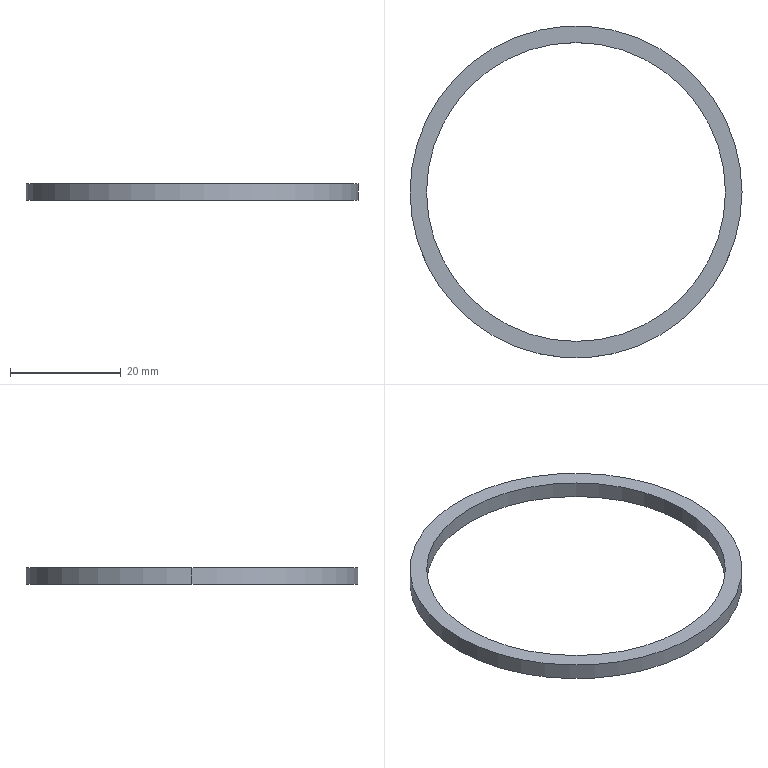Part | SolidWorks | features Extrusion 1 | 1 solid | 6 faces | box 60 x 60 x 3 mm | volume 1612 mm3 | cylinder 4 | plane 2 | commonest cylinder face diameters 54 x2 60 x2
STEP:
#1=CARTESIAN_POINT('',(-27.,0.,3.));
#2=VERTEX_POINT('',#1);
#3=CARTESIAN_POINT('',(27.,0.,3.));
#4=VERTEX_POINT('',#3);
#5=CARTESIAN_POINT('',(0.,0.,3.));
#6=DIRECTION('',(0.,0.,1.));
#7=DIRECTION('',(1.,0.,0.));
#8=AXIS2_PLACEMENT_3D('',#5,#6,#7);
#9=CIRCLE('',#8,27.);
#10=EDGE_CURVE('',#2,#4,#9,.T.);
#11=ORIENTED_EDGE('',*,*,#10,.T.);
#12=CARTESIAN_POINT('',(27.,0.,0.));
#13=VERTEX_POINT('',#12);
#14=CARTESIAN_POINT('',(27.,0.,3.));
#15=DIRECTION('',(0.,0.,-1.));
#16=VECTOR('',#15,1000.);
#17=LINE('',#14,#16);
#18=EDGE_CURVE('',#4,#13,#17,.T.);
#19=ORIENTED_EDGE('',*,*,#18,.T.);
#20=CARTESIAN_POINT('',(-27.,0.,0.));
#21=VERTEX_POINT('',#20);
#22=CARTESIAN_POINT('',(0.,0.,0.));
#23=DIRECTION('',(0.,0.,1.));
#24=DIRECTION('',(1.,0.,0.));
#25=AXIS2_PLACEMENT_3D('',#22,#23,#24);
#26=CIRCLE('',#25,27.);
#27=EDGE_CURVE('',#21,#13,#26,.T.);
#28=ORIENTED_EDGE('',*,*,#27,.F.);
#29=CARTESIAN_POINT('',(-27.,0.,3.));
#30=DIRECTION('',(0.,0.,-1.));
#31=VECTOR('',#30,1000.);
#32=LINE('',#29,#31);
#33=EDGE_CURVE('',#2,#21,#32,.T.);
#34=ORIENTED_EDGE('',*,*,#33,.F.);
#35=EDGE_LOOP('',(#11,#19,#28,#34));
#36=FACE_OUTER_BOUND('',#35,.T.);
#37=CARTESIAN_POINT('',(0.,0.,3.));
#38=DIRECTION('',(0.,0.,-1.));
#39=DIRECTION('',(-1.,0.,0.));
#40=AXIS2_PLACEMENT_3D('',#37,#38,#39);
#41=CYLINDRICAL_SURFACE('',#40,27.);
#42=ADVANCED_FACE('',(#36),#41,.F.);
#43=CARTESIAN_POINT('',(30.,0.,3.));
#44=VERTEX_POINT('',#43);
#45=CARTESIAN_POINT('',(-30.,0.,3.));
#46=VERTEX_POINT('',#45);
#47=CARTESIAN_POINT('',(0.,0.,3.));
#48=DIRECTION('',(0.,0.,1.));
#49=DIRECTION('',(1.,0.,0.));
#50=AXIS2_PLACEMENT_3D('',#47,#48,#49);
#51=CIRCLE('',#50,30.);
#52=EDGE_CURVE('',#44,#46,#51,.T.);
#53=ORIENTED_EDGE('',*,*,#52,.F.);
#54=CARTESIAN_POINT('',(30.,0.,0.));
#55=VERTEX_POINT('',#54);
#56=CARTESIAN_POINT('',(30.,0.,3.));
#57=DIRECTION('',(0.,0.,-1.));
#58=VECTOR('',#57,1000.);
#59=LINE('',#56,#58);
#60=EDGE_CURVE('',#44,#55,#59,.T.);
#61=ORIENTED_EDGE('',*,*,#60,.T.);
#62=CARTESIAN_POINT('',(-30.,0.,0.));
#63=VERTEX_POINT('',#62);
#64=CARTESIAN_POINT('',(0.,0.,0.));
#65=DIRECTION('',(0.,0.,1.));
#66=DIRECTION('',(1.,0.,0.));
#67=AXIS2_PLACEMENT_3D('',#64,#65,#66);
#68=CIRCLE('',#67,30.);
#69=EDGE_CURVE('',#55,#63,#68,.T.);
#70=ORIENTED_EDGE('',*,*,#69,.T.);
#71=CARTESIAN_POINT('',(-30.,0.,3.));
#72=DIRECTION('',(0.,0.,-1.));
#73=VECTOR('',#72,1000.);
#74=LINE('',#71,#73);
#75=EDGE_CURVE('',#46,#63,#74,.T.);
#76=ORIENTED_EDGE('',*,*,#75,.F.);
#77=EDGE_LOOP('',(#53,#61,#70,#76));
#78=FACE_OUTER_BOUND('',#77,.T.);
#79=CARTESIAN_POINT('',(0.,0.,3.));
#80=DIRECTION('',(0.,0.,-1.));
#81=DIRECTION('',(-1.,0.,0.));
#82=AXIS2_PLACEMENT_3D('',#79,#80,#81);
#83=CYLINDRICAL_SURFACE('',#82,30.);
#84=ADVANCED_FACE('',(#78),#83,.T.);
#85=CARTESIAN_POINT('',(0.,0.,3.));
#86=DIRECTION('',(0.,0.,1.));
#87=DIRECTION('',(1.,0.,0.));
#88=AXIS2_PLACEMENT_3D('',#85,#86,#87);
#89=CIRCLE('',#88,30.);
#90=EDGE_CURVE('',#46,#44,#89,.T.);
#91=ORIENTED_EDGE('',*,*,#90,.T.);
#92=ORIENTED_EDGE('',*,*,#52,.T.);
#93=EDGE_LOOP('',(#91,#92));
#94=FACE_OUTER_BOUND('',#93,.T.);
#95=ORIENTED_EDGE('',*,*,#10,.F.);
#96=CARTESIAN_POINT('',(0.,0.,3.));
#97=DIRECTION('',(0.,0.,1.));
#98=DIRECTION('',(1.,0.,0.));
#99=AXIS2_PLACEMENT_3D('',#96,#97,#98);
#100=CIRCLE('',#99,27.);
#101=EDGE_CURVE('',#4,#2,#100,.T.);
#102=ORIENTED_EDGE('',*,*,#101,.F.);
#103=EDGE_LOOP('',(#95,#102));
#104=FACE_BOUND('',#103,.T.);
#105=CARTESIAN_POINT('',(0.,0.,3.));
#106=DIRECTION('',(0.,0.,1.));
#107=DIRECTION('',(1.,0.,0.));
#108=AXIS2_PLACEMENT_3D('',#105,#106,#107);
#109=PLANE('',#108);
#110=ADVANCED_FACE('',(#94,#104),#109,.T.);
#111=CARTESIAN_POINT('',(0.,0.,0.));
#112=DIRECTION('',(0.,0.,1.));
#113=DIRECTION('',(1.,0.,0.));
#114=AXIS2_PLACEMENT_3D('',#111,#112,#113);
#115=CIRCLE('',#114,30.);
#116=EDGE_CURVE('',#63,#55,#115,.T.);
#117=ORIENTED_EDGE('',*,*,#116,.F.);
#118=ORIENTED_EDGE('',*,*,#69,.F.);
#119=EDGE_LOOP('',(#117,#118));
#120=FACE_OUTER_BOUND('',#119,.T.);
#121=ORIENTED_EDGE('',*,*,#27,.T.);
#122=CARTESIAN_POINT('',(0.,0.,0.));
#123=DIRECTION('',(0.,0.,1.));
#124=DIRECTION('',(1.,0.,0.));
#125=AXIS2_PLACEMENT_3D('',#122,#123,#124);
#126=CIRCLE('',#125,27.);
#127=EDGE_CURVE('',#13,#21,#126,.T.);
#128=ORIENTED_EDGE('',*,*,#127,.T.);
#129=EDGE_LOOP('',(#121,#128));
#130=FACE_BOUND('',#129,.T.);
#131=CARTESIAN_POINT('',(0.,0.,0.));
#132=DIRECTION('',(0.,0.,1.));
#133=DIRECTION('',(1.,0.,0.));
#134=AXIS2_PLACEMENT_3D('',#131,#132,#133);
#135=PLANE('',#134);
#136=ADVANCED_FACE('',(#120,#130),#135,.F.);
#137=ORIENTED_EDGE('',*,*,#60,.F.);
#138=ORIENTED_EDGE('',*,*,#90,.F.);
#139=ORIENTED_EDGE('',*,*,#75,.T.);
#140=ORIENTED_EDGE('',*,*,#116,.T.);
#141=EDGE_LOOP('',(#137,#138,#139,#140));
#142=FACE_OUTER_BOUND('',#141,.T.);
#143=CARTESIAN_POINT('',(0.,0.,3.));
#144=DIRECTION('',(0.,0.,-1.));
#145=DIRECTION('',(-1.,0.,0.));
#146=AXIS2_PLACEMENT_3D('',#143,#144,#145);
#147=CYLINDRICAL_SURFACE('',#146,30.);
#148=ADVANCED_FACE('',(#142),#147,.T.);
#149=ORIENTED_EDGE('',*,*,#18,.F.);
#150=ORIENTED_EDGE('',*,*,#101,.T.);
#151=ORIENTED_EDGE('',*,*,#33,.T.);
#152=ORIENTED_EDGE('',*,*,#127,.F.);
#153=EDGE_LOOP('',(#149,#150,#151,#152));
#154=FACE_OUTER_BOUND('',#153,.T.);
#155=CARTESIAN_POINT('',(0.,0.,3.));
#156=DIRECTION('',(0.,0.,-1.));
#157=DIRECTION('',(-1.,0.,0.));
#158=AXIS2_PLACEMENT_3D('',#155,#156,#157);
#159=CYLINDRICAL_SURFACE('',#158,27.);
#160=ADVANCED_FACE('',(#154),#159,.F.);
#161=CLOSED_SHELL('',(#42,#84,#110,#136,#148,#160));
#162=MANIFOLD_SOLID_BREP('',#161);
#163=CARTESIAN_POINT('',(0.,0.,0.));
#164=DIRECTION('',(0.,0.,1.));
#165=DIRECTION('',(1.,0.,0.));
#166=AXIS2_PLACEMENT_3D('',#163,#164,#165);
#167=(LENGTH_UNIT()NAMED_UNIT(*)SI_UNIT(.MILLI.,.METRE.));
#168=UNCERTAINTY_MEASURE_WITH_UNIT(LENGTH_MEASURE(0.00001),#167,'','');
#169=(NAMED_UNIT(*)PLANE_ANGLE_UNIT()SI_UNIT($,.RADIAN.));
#170=(NAMED_UNIT(*)SI_UNIT($,.STERADIAN.)SOLID_ANGLE_UNIT());
#171=(GEOMETRIC_REPRESENTATION_CONTEXT(3)GLOBAL_UNCERTAINTY_ASSIGNED_CONTEXT((#168))GLOBAL_UNIT_ASSIGNED_CONTEXT((#167,#169,#170))REPRESENTATION_CONTEXT('',''));
#172=ADVANCED_BREP_SHAPE_REPRESENTATION('',(#162,#166),#171);